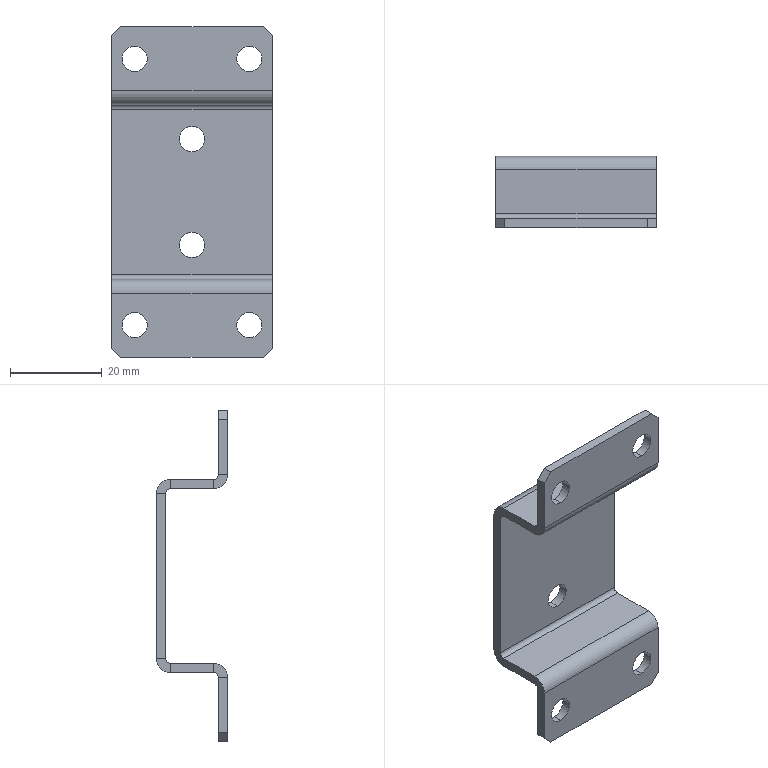Part | STEP file | HXGR200008-06-03-01 | 1 solid | 54 faces | box 35 x 15.5 x 72 mm | volume 6389 mm3 | plane 34 | cylinder 20 | commonest cylinder face diameters 5.5 x12 2 x4 6 x4
STEP:
#1=CARTESIAN_POINT('',(0.,5.75,10.25));
#2=VERTEX_POINT('',#1);
#3=CARTESIAN_POINT('',(0.,5.75,4.75));
#4=VERTEX_POINT('',#3);
#5=CARTESIAN_POINT('',(0.,5.75,7.5));
#6=DIRECTION('',(0.,-1.,0.));
#7=DIRECTION('',(0.,0.,-1.));
#8=AXIS2_PLACEMENT_3D('',#5,#6,#7);
#9=CIRCLE('',#8,2.75);
#10=EDGE_CURVE('',#2,#4,#9,.T.);
#11=ORIENTED_EDGE('',*,*,#10,.T.);
#12=CARTESIAN_POINT('',(0.,7.75,4.75));
#13=VERTEX_POINT('',#12);
#14=CARTESIAN_POINT('',(0.,7.75,4.75));
#15=DIRECTION('',(0.,1.,0.));
#16=VECTOR('',#15,1000.);
#17=LINE('',#14,#16);
#18=EDGE_CURVE('',#4,#13,#17,.T.);
#19=ORIENTED_EDGE('',*,*,#18,.T.);
#20=CARTESIAN_POINT('',(0.,7.75,10.25));
#21=VERTEX_POINT('',#20);
#22=CARTESIAN_POINT('',(0.,7.75,7.5));
#23=DIRECTION('',(0.,1.,0.));
#24=DIRECTION('',(0.,0.,1.));
#25=AXIS2_PLACEMENT_3D('',#22,#23,#24);
#26=CIRCLE('',#25,2.75);
#27=EDGE_CURVE('',#13,#21,#26,.T.);
#28=ORIENTED_EDGE('',*,*,#27,.T.);
#29=CARTESIAN_POINT('',(0.,7.75,10.25));
#30=DIRECTION('',(0.,1.,0.));
#31=VECTOR('',#30,1000.);
#32=LINE('',#29,#31);
#33=EDGE_CURVE('',#2,#21,#32,.T.);
#34=ORIENTED_EDGE('',*,*,#33,.F.);
#35=EDGE_LOOP('',(#11,#19,#28,#34));
#36=FACE_OUTER_BOUND('',#35,.T.);
#37=CARTESIAN_POINT('',(0.,7.75,7.5));
#38=DIRECTION('',(0.,1.,0.));
#39=DIRECTION('',(0.,0.,1.));
#40=AXIS2_PLACEMENT_3D('',#37,#38,#39);
#41=CYLINDRICAL_SURFACE('',#40,2.75);
#42=ADVANCED_FACE('',(#36),#41,.F.);
#43=CARTESIAN_POINT('',(0.,5.75,33.25));
#44=VERTEX_POINT('',#43);
#45=CARTESIAN_POINT('',(0.,5.75,27.75));
#46=VERTEX_POINT('',#45);
#47=CARTESIAN_POINT('',(0.,5.75,30.5));
#48=DIRECTION('',(0.,-1.,0.));
#49=DIRECTION('',(0.,0.,-1.));
#50=AXIS2_PLACEMENT_3D('',#47,#48,#49);
#51=CIRCLE('',#50,2.75);
#52=EDGE_CURVE('',#44,#46,#51,.T.);
#53=ORIENTED_EDGE('',*,*,#52,.T.);
#54=CARTESIAN_POINT('',(0.,7.75,27.75));
#55=VERTEX_POINT('',#54);
#56=CARTESIAN_POINT('',(0.,7.75,27.75));
#57=DIRECTION('',(0.,1.,0.));
#58=VECTOR('',#57,1000.);
#59=LINE('',#56,#58);
#60=EDGE_CURVE('',#46,#55,#59,.T.);
#61=ORIENTED_EDGE('',*,*,#60,.T.);
#62=CARTESIAN_POINT('',(0.,7.75,33.25));
#63=VERTEX_POINT('',#62);
#64=CARTESIAN_POINT('',(0.,7.75,30.5));
#65=DIRECTION('',(0.,1.,0.));
#66=DIRECTION('',(0.,0.,1.));
#67=AXIS2_PLACEMENT_3D('',#64,#65,#66);
#68=CIRCLE('',#67,2.75);
#69=EDGE_CURVE('',#55,#63,#68,.T.);
#70=ORIENTED_EDGE('',*,*,#69,.T.);
#71=CARTESIAN_POINT('',(0.,7.75,33.25));
#72=DIRECTION('',(0.,1.,0.));
#73=VECTOR('',#72,1000.);
#74=LINE('',#71,#73);
#75=EDGE_CURVE('',#44,#63,#74,.T.);
#76=ORIENTED_EDGE('',*,*,#75,.F.);
#77=EDGE_LOOP('',(#53,#61,#70,#76));
#78=FACE_OUTER_BOUND('',#77,.T.);
#79=CARTESIAN_POINT('',(0.,7.75,30.5));
#80=DIRECTION('',(0.,1.,0.));
#81=DIRECTION('',(0.,0.,1.));
#82=AXIS2_PLACEMENT_3D('',#79,#80,#81);
#83=CYLINDRICAL_SURFACE('',#82,2.75);
#84=ADVANCED_FACE('',(#78),#83,.F.);
#85=CARTESIAN_POINT('',(-12.5,-7.75,-7.25));
#86=VERTEX_POINT('',#85);
#87=CARTESIAN_POINT('',(-12.5,-7.75,-12.75));
#88=VERTEX_POINT('',#87);
#89=CARTESIAN_POINT('',(-12.5,-7.75,-10.));
#90=DIRECTION('',(0.,-1.,0.));
#91=DIRECTION('',(0.,0.,-1.));
#92=AXIS2_PLACEMENT_3D('',#89,#90,#91);
#93=CIRCLE('',#92,2.75);
#94=EDGE_CURVE('',#86,#88,#93,.T.);
#95=ORIENTED_EDGE('',*,*,#94,.T.);
#96=CARTESIAN_POINT('',(-12.5,-5.75,-12.75));
#97=VERTEX_POINT('',#96);
#98=CARTESIAN_POINT('',(-12.5,-5.75,-12.75));
#99=DIRECTION('',(0.,1.,0.));
#100=VECTOR('',#99,1000.);
#101=LINE('',#98,#100);
#102=EDGE_CURVE('',#88,#97,#101,.T.);
#103=ORIENTED_EDGE('',*,*,#102,.T.);
#104=CARTESIAN_POINT('',(-12.5,-5.75,-7.25));
#105=VERTEX_POINT('',#104);
#106=CARTESIAN_POINT('',(-12.5,-5.75,-10.));
#107=DIRECTION('',(0.,1.,0.));
#108=DIRECTION('',(0.,0.,1.));
#109=AXIS2_PLACEMENT_3D('',#106,#107,#108);
#110=CIRCLE('',#109,2.75);
#111=EDGE_CURVE('',#97,#105,#110,.T.);
#112=ORIENTED_EDGE('',*,*,#111,.T.);
#113=CARTESIAN_POINT('',(-12.5,-5.75,-7.25));
#114=DIRECTION('',(0.,1.,0.));
#115=VECTOR('',#114,1000.);
#116=LINE('',#113,#115);
#117=EDGE_CURVE('',#86,#105,#116,.T.);
#118=ORIENTED_EDGE('',*,*,#117,.F.);
#119=EDGE_LOOP('',(#95,#103,#112,#118));
#120=FACE_OUTER_BOUND('',#119,.T.);
#121=CARTESIAN_POINT('',(-12.5,-5.75,-10.));
#122=DIRECTION('',(0.,1.,0.));
#123=DIRECTION('',(0.,0.,1.));
#124=AXIS2_PLACEMENT_3D('',#121,#122,#123);
#125=CYLINDRICAL_SURFACE('',#124,2.75);
#126=ADVANCED_FACE('',(#120),#125,.F.);
#127=CARTESIAN_POINT('',(12.5,-7.75,-7.25));
#128=VERTEX_POINT('',#127);
#129=CARTESIAN_POINT('',(12.5,-7.75,-12.75));
#130=VERTEX_POINT('',#129);
#131=CARTESIAN_POINT('',(12.5,-7.75,-10.));
#132=DIRECTION('',(0.,-1.,0.));
#133=DIRECTION('',(0.,0.,-1.));
#134=AXIS2_PLACEMENT_3D('',#131,#132,#133);
#135=CIRCLE('',#134,2.75);
#136=EDGE_CURVE('',#128,#130,#135,.T.);
#137=ORIENTED_EDGE('',*,*,#136,.T.);
#138=CARTESIAN_POINT('',(12.5,-5.75,-12.75));
#139=VERTEX_POINT('',#138);
#140=CARTESIAN_POINT('',(12.5,-5.75,-12.75));
#141=DIRECTION('',(0.,1.,0.));
#142=VECTOR('',#141,1000.);
#143=LINE('',#140,#142);
#144=EDGE_CURVE('',#130,#139,#143,.T.);
#145=ORIENTED_EDGE('',*,*,#144,.T.);
#146=CARTESIAN_POINT('',(12.5,-5.75,-7.25));
#147=VERTEX_POINT('',#146);
#148=CARTESIAN_POINT('',(12.5,-5.75,-10.));
#149=DIRECTION('',(0.,1.,0.));
#150=DIRECTION('',(0.,0.,1.));
#151=AXIS2_PLACEMENT_3D('',#148,#149,#150);
#152=CIRCLE('',#151,2.75);
#153=EDGE_CURVE('',#139,#147,#152,.T.);
#154=ORIENTED_EDGE('',*,*,#153,.T.);
#155=CARTESIAN_POINT('',(12.5,-5.75,-7.25));
#156=DIRECTION('',(0.,1.,0.));
#157=VECTOR('',#156,1000.);
#158=LINE('',#155,#157);
#159=EDGE_CURVE('',#128,#147,#158,.T.);
#160=ORIENTED_EDGE('',*,*,#159,.F.);
#161=EDGE_LOOP('',(#137,#145,#154,#160));
#162=FACE_OUTER_BOUND('',#161,.T.);
#163=CARTESIAN_POINT('',(12.5,-5.75,-10.));
#164=DIRECTION('',(0.,1.,0.));
#165=DIRECTION('',(0.,0.,1.));
#166=AXIS2_PLACEMENT_3D('',#163,#164,#165);
#167=CYLINDRICAL_SURFACE('',#166,2.75);
#168=ADVANCED_FACE('',(#162),#167,.F.);
#169=CARTESIAN_POINT('',(-12.5,-7.75,45.25));
#170=VERTEX_POINT('',#169);
#171=CARTESIAN_POINT('',(-12.5,-7.75,50.75));
#172=VERTEX_POINT('',#171);
#173=CARTESIAN_POINT('',(-12.5,-7.75,48.));
#174=DIRECTION('',(0.,1.,0.));
#175=DIRECTION('',(0.,0.,1.));
#176=AXIS2_PLACEMENT_3D('',#173,#174,#175);
#177=CIRCLE('',#176,2.75);
#178=EDGE_CURVE('',#170,#172,#177,.T.);
#179=ORIENTED_EDGE('',*,*,#178,.F.);
#180=CARTESIAN_POINT('',(-12.5,-5.75,45.25));
#181=VERTEX_POINT('',#180);
#182=CARTESIAN_POINT('',(-12.5,-5.75,45.25));
#183=DIRECTION('',(0.,1.,0.));
#184=VECTOR('',#183,1000.);
#185=LINE('',#182,#184);
#186=EDGE_CURVE('',#170,#181,#185,.T.);
#187=ORIENTED_EDGE('',*,*,#186,.T.);
#188=CARTESIAN_POINT('',(-12.5,-5.75,50.75));
#189=VERTEX_POINT('',#188);
#190=CARTESIAN_POINT('',(-12.5,-5.75,48.));
#191=DIRECTION('',(0.,1.,0.));
#192=DIRECTION('',(0.,0.,1.));
#193=AXIS2_PLACEMENT_3D('',#190,#191,#192);
#194=CIRCLE('',#193,2.75);
#195=EDGE_CURVE('',#181,#189,#194,.T.);
#196=ORIENTED_EDGE('',*,*,#195,.T.);
#197=CARTESIAN_POINT('',(-12.5,-5.75,50.75));
#198=DIRECTION('',(0.,1.,0.));
#199=VECTOR('',#198,1000.);
#200=LINE('',#197,#199);
#201=EDGE_CURVE('',#172,#189,#200,.T.);
#202=ORIENTED_EDGE('',*,*,#201,.F.);
#203=EDGE_LOOP('',(#179,#187,#196,#202));
#204=FACE_OUTER_BOUND('',#203,.T.);
#205=CARTESIAN_POINT('',(-12.5,-5.75,48.));
#206=DIRECTION('',(0.,1.,0.));
#207=DIRECTION('',(0.,0.,1.));
#208=AXIS2_PLACEMENT_3D('',#205,#206,#207);
#209=CYLINDRICAL_SURFACE('',#208,2.75);
#210=ADVANCED_FACE('',(#204),#209,.F.);
#211=CARTESIAN_POINT('',(12.5,-7.75,45.25));
#212=VERTEX_POINT('',#211);
#213=CARTESIAN_POINT('',(12.5,-7.75,50.75));
#214=VERTEX_POINT('',#213);
#215=CARTESIAN_POINT('',(12.5,-7.75,48.));
#216=DIRECTION('',(0.,1.,0.));
#217=DIRECTION('',(0.,0.,1.));
#218=AXIS2_PLACEMENT_3D('',#215,#216,#217);
#219=CIRCLE('',#218,2.75);
#220=EDGE_CURVE('',#212,#214,#219,.T.);
#221=ORIENTED_EDGE('',*,*,#220,.F.);
#222=CARTESIAN_POINT('',(12.5,-5.75,45.25));
#223=VERTEX_POINT('',#222);
#224=CARTESIAN_POINT('',(12.5,-5.75,45.25));
#225=DIRECTION('',(0.,1.,0.));
#226=VECTOR('',#225,1000.);
#227=LINE('',#224,#226);
#228=EDGE_CURVE('',#212,#223,#227,.T.);
#229=ORIENTED_EDGE('',*,*,#228,.T.);
#230=CARTESIAN_POINT('',(12.5,-5.75,50.75));
#231=VERTEX_POINT('',#230);
#232=CARTESIAN_POINT('',(12.5,-5.75,48.));
#233=DIRECTION('',(0.,1.,0.));
#234=DIRECTION('',(0.,0.,1.));
#235=AXIS2_PLACEMENT_3D('',#232,#233,#234);
#236=CIRCLE('',#235,2.75);
#237=EDGE_CURVE('',#223,#231,#236,.T.);
#238=ORIENTED_EDGE('',*,*,#237,.T.);
#239=CARTESIAN_POINT('',(12.5,-5.75,50.75));
#240=DIRECTION('',(0.,1.,0.));
#241=VECTOR('',#240,1000.);
#242=LINE('',#239,#241);
#243=EDGE_CURVE('',#214,#231,#242,.T.);
#244=ORIENTED_EDGE('',*,*,#243,.F.);
#245=EDGE_LOOP('',(#221,#229,#238,#244));
#246=FACE_OUTER_BOUND('',#245,.T.);
#247=CARTESIAN_POINT('',(12.5,-5.75,48.));
#248=DIRECTION('',(0.,1.,0.));
#249=DIRECTION('',(0.,0.,1.));
#250=AXIS2_PLACEMENT_3D('',#247,#248,#249);
#251=CYLINDRICAL_SURFACE('',#250,2.75);
#252=ADVANCED_FACE('',(#246),#251,.F.);
#253=CARTESIAN_POINT('',(-12.5,-5.75,-10.));
#254=DIRECTION('',(0.,1.,0.));
#255=DIRECTION('',(0.,0.,1.));
#256=AXIS2_PLACEMENT_3D('',#253,#254,#255);
#257=CIRCLE('',#256,2.75);
#258=EDGE_CURVE('',#105,#97,#257,.T.);
#259=ORIENTED_EDGE('',*,*,#258,.F.);
#260=ORIENTED_EDGE('',*,*,#111,.F.);
#261=EDGE_LOOP('',(#259,#260));
#262=FACE_BOUND('',#261,.T.);
#263=CARTESIAN_POINT('',(15.5,-5.75,-17.));
#264=VERTEX_POINT('',#263);
#265=CARTESIAN_POINT('',(-15.5,-5.75,-17.));
#266=VERTEX_POINT('',#265);
#267=CARTESIAN_POINT('',(0.,-5.75,-17.));
#268=DIRECTION('',(-1.,0.,0.));
#269=VECTOR('',#268,1000.);
#270=LINE('',#267,#269);
#271=EDGE_CURVE('',#264,#266,#270,.T.);
#272=ORIENTED_EDGE('',*,*,#271,.T.);
#273=CARTESIAN_POINT('',(-17.5,-5.75,-15.));
#274=VERTEX_POINT('',#273);
#275=CARTESIAN_POINT('',(-15.5,-5.75,-17.));
#276=DIRECTION('',(-0.7071,0.,0.7071));
#277=VECTOR('',#276,1000.);
#278=LINE('',#275,#277);
#279=EDGE_CURVE('',#266,#274,#278,.T.);
#280=ORIENTED_EDGE('',*,*,#279,.T.);
#281=CARTESIAN_POINT('',(-17.5,-5.75,-3.));
#282=VERTEX_POINT('',#281);
#283=CARTESIAN_POINT('',(-17.5,-5.75,0.));
#284=DIRECTION('',(0.,0.,1.));
#285=VECTOR('',#284,1000.);
#286=LINE('',#283,#285);
#287=EDGE_CURVE('',#274,#282,#286,.T.);
#288=ORIENTED_EDGE('',*,*,#287,.T.);
#289=CARTESIAN_POINT('',(17.5,-5.75,-3.));
#290=VERTEX_POINT('',#289);
#291=CARTESIAN_POINT('',(17.5,-5.75,-3.));
#292=DIRECTION('',(-1.,0.,0.));
#293=VECTOR('',#292,1000.);
#294=LINE('',#291,#293);
#295=EDGE_CURVE('',#290,#282,#294,.T.);
#296=ORIENTED_EDGE('',*,*,#295,.F.);
#297=CARTESIAN_POINT('',(17.5,-5.75,-15.));
#298=VERTEX_POINT('',#297);
#299=CARTESIAN_POINT('',(17.5,-5.75,0.));
#300=DIRECTION('',(0.,0.,-1.));
#301=VECTOR('',#300,1000.);
#302=LINE('',#299,#301);
#303=EDGE_CURVE('',#290,#298,#302,.T.);
#304=ORIENTED_EDGE('',*,*,#303,.T.);
#305=CARTESIAN_POINT('',(17.5,-5.75,-15.));
#306=DIRECTION('',(-0.7071,0.,-0.7071));
#307=VECTOR('',#306,1000.);
#308=LINE('',#305,#307);
#309=EDGE_CURVE('',#298,#264,#308,.T.);
#310=ORIENTED_EDGE('',*,*,#309,.T.);
#311=EDGE_LOOP('',(#272,#280,#288,#296,#304,#310));
#312=FACE_OUTER_BOUND('',#311,.T.);
#313=CARTESIAN_POINT('',(12.5,-5.75,-10.));
#314=DIRECTION('',(0.,1.,0.));
#315=DIRECTION('',(0.,0.,1.));
#316=AXIS2_PLACEMENT_3D('',#313,#314,#315);
#317=CIRCLE('',#316,2.75);
#318=EDGE_CURVE('',#147,#139,#317,.T.);
#319=ORIENTED_EDGE('',*,*,#318,.F.);
#320=ORIENTED_EDGE('',*,*,#153,.F.);
#321=EDGE_LOOP('',(#319,#320));
#322=FACE_BOUND('',#321,.T.);
#323=CARTESIAN_POINT('',(0.,-5.75,0.));
#324=DIRECTION('',(0.,-1.,0.));
#325=DIRECTION('',(0.,0.,-1.));
#326=AXIS2_PLACEMENT_3D('',#323,#324,#325);
#327=PLANE('',#326);
#328=ADVANCED_FACE('',(#262,#312,#322),#327,.F.);
#329=CARTESIAN_POINT('',(-17.5,-4.75,40.));
#330=VERTEX_POINT('',#329);
#331=CARTESIAN_POINT('',(-17.5,-4.75,38.));
#332=VERTEX_POINT('',#331);
#333=CARTESIAN_POINT('',(-17.5,-4.75,40.));
#334=DIRECTION('',(0.,0.,-1.));
#335=VECTOR('',#334,1000.);
#336=LINE('',#333,#335);
#337=EDGE_CURVE('',#330,#332,#336,.T.);
#338=ORIENTED_EDGE('',*,*,#337,.F.);
#339=CARTESIAN_POINT('',(-17.5,4.75,40.));
#340=VERTEX_POINT('',#339);
#341=CARTESIAN_POINT('',(-17.5,0.,40.));
#342=DIRECTION('',(0.,-1.,0.));
#343=VECTOR('',#342,1000.);
#344=LINE('',#341,#343);
#345=EDGE_CURVE('',#340,#330,#344,.T.);
#346=ORIENTED_EDGE('',*,*,#345,.F.);
#347=CARTESIAN_POINT('',(-17.5,4.75,38.));
#348=VERTEX_POINT('',#347);
#349=CARTESIAN_POINT('',(-17.5,4.75,38.));
#350=DIRECTION('',(0.,0.,1.));
#351=VECTOR('',#350,1000.);
#352=LINE('',#349,#351);
#353=EDGE_CURVE('',#348,#340,#352,.T.);
#354=ORIENTED_EDGE('',*,*,#353,.F.);
#355=CARTESIAN_POINT('',(-17.5,-7.75,38.));
#356=DIRECTION('',(0.,-1.,0.));
#357=VECTOR('',#356,1000.);
#358=LINE('',#355,#357);
#359=EDGE_CURVE('',#348,#332,#358,.T.);
#360=ORIENTED_EDGE('',*,*,#359,.T.);
#361=EDGE_LOOP('',(#338,#346,#354,#360));
#362=FACE_OUTER_BOUND('',#361,.T.);
#363=CARTESIAN_POINT('',(-17.5,-7.75,40.));
#364=DIRECTION('',(1.,0.,0.));
#365=DIRECTION('',(0.,0.,-1.));
#366=AXIS2_PLACEMENT_3D('',#363,#364,#365);
#367=PLANE('',#366);
#368=ADVANCED_FACE('',(#362),#367,.F.);
#369=CARTESIAN_POINT('',(17.5,-4.75,40.));
#370=VERTEX_POINT('',#369);
#371=CARTESIAN_POINT('',(17.5,-4.75,38.));
#372=VERTEX_POINT('',#371);
#373=CARTESIAN_POINT('',(17.5,-4.75,40.));
#374=DIRECTION('',(0.,0.,-1.));
#375=VECTOR('',#374,1000.);
#376=LINE('',#373,#375);
#377=EDGE_CURVE('',#370,#372,#376,.T.);
#378=ORIENTED_EDGE('',*,*,#377,.T.);
#379=CARTESIAN_POINT('',(17.5,4.75,38.));
#380=VERTEX_POINT('',#379);
#381=CARTESIAN_POINT('',(17.5,5.75,38.));
#382=DIRECTION('',(0.,1.,0.));
#383=VECTOR('',#382,1000.);
#384=LINE('',#381,#383);
#385=EDGE_CURVE('',#372,#380,#384,.T.);
#386=ORIENTED_EDGE('',*,*,#385,.T.);
#387=CARTESIAN_POINT('',(17.5,4.75,40.));
#388=VERTEX_POINT('',#387);
#389=CARTESIAN_POINT('',(17.5,4.75,40.));
#390=DIRECTION('',(0.,0.,1.));
#391=VECTOR('',#390,1000.);
#392=LINE('',#389,#391);
#393=EDGE_CURVE('',#380,#388,#392,.T.);
#394=ORIENTED_EDGE('',*,*,#393,.T.);
#395=CARTESIAN_POINT('',(17.5,0.,40.));
#396=DIRECTION('',(0.,1.,0.));
#397=VECTOR('',#396,1000.);
#398=LINE('',#395,#397);
#399=EDGE_CURVE('',#370,#388,#398,.T.);
#400=ORIENTED_EDGE('',*,*,#399,.F.);
#401=EDGE_LOOP('',(#378,#386,#394,#400));
#402=FACE_OUTER_BOUND('',#401,.T.);
#403=CARTESIAN_POINT('',(17.5,5.75,40.));
#404=DIRECTION('',(-1.,0.,0.));
#405=DIRECTION('',(0.,0.,1.));
#406=AXIS2_PLACEMENT_3D('',#403,#404,#405);
#407=PLANE('',#406);
#408=ADVANCED_FACE('',(#402),#407,.F.);
#409=CARTESIAN_POINT('',(17.5,-4.75,40.));
#410=DIRECTION('',(-1.,0.,0.));
#411=VECTOR('',#410,1000.);
#412=LINE('',#409,#411);
#413=EDGE_CURVE('',#370,#330,#412,.T.);
#414=ORIENTED_EDGE('',*,*,#413,.F.);
#415=ORIENTED_EDGE('',*,*,#399,.T.);
#416=CARTESIAN_POINT('',(17.5,4.75,40.));
#417=DIRECTION('',(1.,0.,0.));
#418=VECTOR('',#417,1000.);
#419=LINE('',#416,#418);
#420=EDGE_CURVE('',#340,#388,#419,.T.);
#421=ORIENTED_EDGE('',*,*,#420,.F.);
#422=ORIENTED_EDGE('',*,*,#345,.T.);
#423=EDGE_LOOP('',(#414,#415,#421,#422));
#424=FACE_OUTER_BOUND('',#423,.T.);
#425=CARTESIAN_POINT('',(0.,0.,40.));
#426=DIRECTION('',(0.,0.,-1.));
#427=DIRECTION('',(0.,1.,0.));
#428=AXIS2_PLACEMENT_3D('',#425,#426,#427);
#429=PLANE('',#428);
#430=ADVANCED_FACE('',(#424),#429,.F.);
#431=ORIENTED_EDGE('',*,*,#385,.F.);
#432=CARTESIAN_POINT('',(17.5,-4.75,38.));
#433=DIRECTION('',(-1.,0.,0.));
#434=VECTOR('',#433,1000.);
#435=LINE('',#432,#434);
#436=EDGE_CURVE('',#372,#332,#435,.T.);
#437=ORIENTED_EDGE('',*,*,#436,.T.);
#438=ORIENTED_EDGE('',*,*,#359,.F.);
#439=CARTESIAN_POINT('',(17.5,4.75,38.));
#440=DIRECTION('',(-1.,0.,0.));
#441=VECTOR('',#440,1000.);
#442=LINE('',#439,#441);
#443=EDGE_CURVE('',#380,#348,#442,.T.);
#444=ORIENTED_EDGE('',*,*,#443,.F.);
#445=EDGE_LOOP('',(#431,#437,#438,#444));
#446=FACE_OUTER_BOUND('',#445,.T.);
#447=CARTESIAN_POINT('',(0.,0.,38.));
#448=DIRECTION('',(0.,0.,-1.));
#449=DIRECTION('',(0.,1.,0.));
#450=AXIS2_PLACEMENT_3D('',#447,#448,#449);
#451=PLANE('',#450);
#452=ADVANCED_FACE('',(#446),#451,.T.);
#453=CARTESIAN_POINT('',(17.5,5.75,37.));
#454=VERTEX_POINT('',#453);
#455=CARTESIAN_POINT('',(17.5,7.75,37.));
#456=VERTEX_POINT('',#455);
#457=CARTESIAN_POINT('',(17.5,5.75,37.));
#458=DIRECTION('',(0.,1.,0.));
#459=VECTOR('',#458,1000.);
#460=LINE('',#457,#459);
#461=EDGE_CURVE('',#454,#456,#460,.T.);
#462=ORIENTED_EDGE('',*,*,#461,.F.);
#463=CARTESIAN_POINT('',(17.5,5.75,1.));
#464=VERTEX_POINT('',#463);
#465=CARTESIAN_POINT('',(17.5,5.75,0.));
#466=DIRECTION('',(0.,0.,-1.));
#467=VECTOR('',#466,1000.);
#468=LINE('',#465,#467);
#469=EDGE_CURVE('',#454,#464,#468,.T.);
#470=ORIENTED_EDGE('',*,*,#469,.T.);
#471=CARTESIAN_POINT('',(17.5,7.75,1.));
#472=VERTEX_POINT('',#471);
#473=CARTESIAN_POINT('',(17.5,7.75,1.));
#474=DIRECTION('',(0.,1.,0.));
#475=VECTOR('',#474,1000.);
#476=LINE('',#473,#475);
#477=EDGE_CURVE('',#464,#472,#476,.T.);
#478=ORIENTED_EDGE('',*,*,#477,.T.);
#479=CARTESIAN_POINT('',(17.5,7.75,0.));
#480=DIRECTION('',(0.,0.,-1.));
#481=VECTOR('',#480,1000.);
#482=LINE('',#479,#481);
#483=EDGE_CURVE('',#456,#472,#482,.T.);
#484=ORIENTED_EDGE('',*,*,#483,.F.);
#485=EDGE_LOOP('',(#462,#470,#478,#484));
#486=FACE_OUTER_BOUND('',#485,.T.);
#487=CARTESIAN_POINT('',(17.5,7.75,0.));
#488=DIRECTION('',(-1.,0.,0.));
#489=DIRECTION('',(0.,0.,1.));
#490=AXIS2_PLACEMENT_3D('',#487,#488,#489);
#491=PLANE('',#490);
#492=ADVANCED_FACE('',(#486),#491,.F.);
#493=CARTESIAN_POINT('',(-17.5,5.75,37.));
#494=VERTEX_POINT('',#493);
#495=CARTESIAN_POINT('',(-17.5,7.75,37.));
#496=VERTEX_POINT('',#495);
#497=CARTESIAN_POINT('',(-17.5,5.75,37.));
#498=DIRECTION('',(0.,1.,0.));
#499=VECTOR('',#498,1000.);
#500=LINE('',#497,#499);
#501=EDGE_CURVE('',#494,#496,#500,.T.);
#502=ORIENTED_EDGE('',*,*,#501,.T.);
#503=CARTESIAN_POINT('',(-17.5,7.75,1.));
#504=VERTEX_POINT('',#503);
#505=CARTESIAN_POINT('',(-17.5,7.75,0.));
#506=DIRECTION('',(0.,0.,1.));
#507=VECTOR('',#506,1000.);
#508=LINE('',#505,#507);
#509=EDGE_CURVE('',#504,#496,#508,.T.);
#510=ORIENTED_EDGE('',*,*,#509,.F.);
#511=CARTESIAN_POINT('',(-17.5,5.75,1.));
#512=VERTEX_POINT('',#511);
#513=CARTESIAN_POINT('',(-17.5,5.75,1.));
#514=DIRECTION('',(0.,1.,0.));
#515=VECTOR('',#514,1000.);
#516=LINE('',#513,#515);
#517=EDGE_CURVE('',#512,#504,#516,.T.);
#518=ORIENTED_EDGE('',*,*,#517,.F.);
#519=CARTESIAN_POINT('',(-17.5,5.75,40.));
#520=DIRECTION('',(0.,0.,1.));
#521=VECTOR('',#520,1000.);
#522=LINE('',#519,#521);
#523=EDGE_CURVE('',#512,#494,#522,.T.);
#524=ORIENTED_EDGE('',*,*,#523,.T.);
#525=EDGE_LOOP('',(#502,#510,#518,#524));
#526=FACE_OUTER_BOUND('',#525,.T.);
#527=CARTESIAN_POINT('',(-17.5,7.75,40.));
#528=DIRECTION('',(1.,0.,0.));
#529=DIRECTION('',(0.,0.,-1.));
#530=AXIS2_PLACEMENT_3D('',#527,#528,#529);
#531=PLANE('',#530);
#532=ADVANCED_FACE('',(#526),#531,.F.);
#533=CARTESIAN_POINT('',(0.,7.75,7.5));
#534=DIRECTION('',(0.,1.,0.));
#535=DIRECTION('',(0.,0.,1.));
#536=AXIS2_PLACEMENT_3D('',#533,#534,#535);
#537=CIRCLE('',#536,2.75);
#538=EDGE_CURVE('',#21,#13,#537,.T.);
#539=ORIENTED_EDGE('',*,*,#538,.F.);
#540=ORIENTED_EDGE('',*,*,#27,.F.);
#541=EDGE_LOOP('',(#539,#540));
#542=FACE_BOUND('',#541,.T.);
#543=CARTESIAN_POINT('',(0.,7.75,30.5));
#544=DIRECTION('',(0.,1.,0.));
#545=DIRECTION('',(0.,0.,1.));
#546=AXIS2_PLACEMENT_3D('',#543,#544,#545);
#547=CIRCLE('',#546,2.75);
#548=EDGE_CURVE('',#63,#55,#547,.T.);
#549=ORIENTED_EDGE('',*,*,#548,.F.);
#550=ORIENTED_EDGE('',*,*,#69,.F.);
#551=EDGE_LOOP('',(#549,#550));
#552=FACE_BOUND('',#551,.T.);
#553=CARTESIAN_POINT('',(-17.5,7.75,37.));
#554=DIRECTION('',(1.,0.,0.));
#555=VECTOR('',#554,1000.);
#556=LINE('',#553,#555);
#557=EDGE_CURVE('',#496,#456,#556,.T.);
#558=ORIENTED_EDGE('',*,*,#557,.T.);
#559=ORIENTED_EDGE('',*,*,#483,.T.);
#560=CARTESIAN_POINT('',(17.5,7.75,1.));
#561=DIRECTION('',(1.,0.,0.));
#562=VECTOR('',#561,1000.);
#563=LINE('',#560,#562);
#564=EDGE_CURVE('',#504,#472,#563,.T.);
#565=ORIENTED_EDGE('',*,*,#564,.F.);
#566=ORIENTED_EDGE('',*,*,#509,.T.);
#567=EDGE_LOOP('',(#558,#559,#565,#566));
#568=FACE_OUTER_BOUND('',#567,.T.);
#569=CARTESIAN_POINT('',(0.,7.75,0.));
#570=DIRECTION('',(0.,-1.,0.));
#571=DIRECTION('',(0.,0.,-1.));
#572=AXIS2_PLACEMENT_3D('',#569,#570,#571);
#573=PLANE('',#572);
#574=ADVANCED_FACE('',(#542,#552,#568),#573,.F.);
#575=ORIENTED_EDGE('',*,*,#10,.F.);
#576=CARTESIAN_POINT('',(0.,5.75,7.5));
#577=DIRECTION('',(0.,-1.,0.));
#578=DIRECTION('',(0.,0.,-1.));
#579=AXIS2_PLACEMENT_3D('',#576,#577,#578);
#580=CIRCLE('',#579,2.75);
#581=EDGE_CURVE('',#4,#2,#580,.T.);
#582=ORIENTED_EDGE('',*,*,#581,.F.);
#583=EDGE_LOOP('',(#575,#582));
#584=FACE_BOUND('',#583,.T.);
#585=ORIENTED_EDGE('',*,*,#52,.F.);
#586=CARTESIAN_POINT('',(0.,5.75,30.5));
#587=DIRECTION('',(0.,-1.,0.));
#588=DIRECTION('',(0.,0.,-1.));
#589=AXIS2_PLACEMENT_3D('',#586,#587,#588);
#590=CIRCLE('',#589,2.75);
#591=EDGE_CURVE('',#46,#44,#590,.T.);
#592=ORIENTED_EDGE('',*,*,#591,.F.);
#593=EDGE_LOOP('',(#585,#592));
#594=FACE_BOUND('',#593,.T.);
#595=ORIENTED_EDGE('',*,*,#469,.F.);
#596=CARTESIAN_POINT('',(-17.5,5.75,37.));
#597=DIRECTION('',(1.,0.,0.));
#598=VECTOR('',#597,1000.);
#599=LINE('',#596,#598);
#600=EDGE_CURVE('',#494,#454,#599,.T.);
#601=ORIENTED_EDGE('',*,*,#600,.F.);
#602=ORIENTED_EDGE('',*,*,#523,.F.);
#603=CARTESIAN_POINT('',(17.5,5.75,1.));
#604=DIRECTION('',(-1.,0.,0.));
#605=VECTOR('',#604,1000.);
#606=LINE('',#603,#605);
#607=EDGE_CURVE('',#464,#512,#606,.T.);
#608=ORIENTED_EDGE('',*,*,#607,.F.);
#609=EDGE_LOOP('',(#595,#601,#602,#608));
#610=FACE_OUTER_BOUND('',#609,.T.);
#611=CARTESIAN_POINT('',(0.,5.75,0.));
#612=DIRECTION('',(0.,-1.,0.));
#613=DIRECTION('',(0.,0.,-1.));
#614=AXIS2_PLACEMENT_3D('',#611,#612,#613);
#615=PLANE('',#614);
#616=ADVANCED_FACE('',(#584,#594,#610),#615,.T.);
#617=CARTESIAN_POINT('',(-17.5,4.75,0.));
#618=VERTEX_POINT('',#617);
#619=CARTESIAN_POINT('',(-17.5,-4.75,0.));
#620=VERTEX_POINT('',#619);
#621=CARTESIAN_POINT('',(-17.5,7.75,0.));
#622=DIRECTION('',(0.,-1.,0.));
#623=VECTOR('',#622,1000.);
#624=LINE('',#621,#623);
#625=EDGE_CURVE('',#618,#620,#624,.T.);
#626=ORIENTED_EDGE('',*,*,#625,.F.);
#627=CARTESIAN_POINT('',(-17.5,4.75,-2.));
#628=VERTEX_POINT('',#627);
#629=CARTESIAN_POINT('',(-17.5,4.75,0.));
#630=DIRECTION('',(0.,0.,-1.));
#631=VECTOR('',#630,1000.);
#632=LINE('',#629,#631);
#633=EDGE_CURVE('',#618,#628,#632,.T.);
#634=ORIENTED_EDGE('',*,*,#633,.T.);
#635=CARTESIAN_POINT('',(-17.5,-4.75,-2.));
#636=VERTEX_POINT('',#635);
#637=CARTESIAN_POINT('',(-17.5,7.75,-2.));
#638=DIRECTION('',(0.,-1.,0.));
#639=VECTOR('',#638,1000.);
#640=LINE('',#637,#639);
#641=EDGE_CURVE('',#628,#636,#640,.T.);
#642=ORIENTED_EDGE('',*,*,#641,.T.);
#643=CARTESIAN_POINT('',(-17.5,-4.75,-2.));
#644=DIRECTION('',(0.,0.,1.));
#645=VECTOR('',#644,1000.);
#646=LINE('',#643,#645);
#647=EDGE_CURVE('',#636,#620,#646,.T.);
#648=ORIENTED_EDGE('',*,*,#647,.T.);
#649=EDGE_LOOP('',(#626,#634,#642,#648));
#650=FACE_OUTER_BOUND('',#649,.T.);
#651=CARTESIAN_POINT('',(-17.5,7.75,-2.));
#652=DIRECTION('',(-1.,0.,0.));
#653=DIRECTION('',(0.,-1.,0.));
#654=AXIS2_PLACEMENT_3D('',#651,#652,#653);
#655=PLANE('',#654);
#656=ADVANCED_FACE('',(#650),#655,.T.);
#657=CARTESIAN_POINT('',(17.5,4.75,-2.));
#658=VERTEX_POINT('',#657);
#659=CARTESIAN_POINT('',(-17.5,4.75,-2.));
#660=DIRECTION('',(1.,0.,0.));
#661=VECTOR('',#660,1000.);
#662=LINE('',#659,#661);
#663=EDGE_CURVE('',#628,#658,#662,.T.);
#664=ORIENTED_EDGE('',*,*,#663,.T.);
#665=CARTESIAN_POINT('',(17.5,-4.75,-2.));
#666=VERTEX_POINT('',#665);
#667=CARTESIAN_POINT('',(17.5,7.75,-2.));
#668=DIRECTION('',(0.,1.,0.));
#669=VECTOR('',#668,1000.);
#670=LINE('',#667,#669);
#671=EDGE_CURVE('',#666,#658,#670,.T.);
#672=ORIENTED_EDGE('',*,*,#671,.F.);
#673=CARTESIAN_POINT('',(-17.5,-4.75,-2.));
#674=DIRECTION('',(1.,0.,0.));
#675=VECTOR('',#674,1000.);
#676=LINE('',#673,#675);
#677=EDGE_CURVE('',#636,#666,#676,.T.);
#678=ORIENTED_EDGE('',*,*,#677,.F.);
#679=ORIENTED_EDGE('',*,*,#641,.F.);
#680=EDGE_LOOP('',(#664,#672,#678,#679));
#681=FACE_OUTER_BOUND('',#680,.T.);
#682=CARTESIAN_POINT('',(0.,0.,-2.));
#683=DIRECTION('',(0.,0.,1.));
#684=DIRECTION('',(1.,0.,0.));
#685=AXIS2_PLACEMENT_3D('',#682,#683,#684);
#686=PLANE('',#685);
#687=ADVANCED_FACE('',(#681),#686,.F.);
#688=CARTESIAN_POINT('',(17.5,-4.75,0.));
#689=VERTEX_POINT('',#688);
#690=CARTESIAN_POINT('',(17.5,4.75,0.));
#691=VERTEX_POINT('',#690);
#692=CARTESIAN_POINT('',(17.5,7.75,0.));
#693=DIRECTION('',(0.,1.,0.));
#694=VECTOR('',#693,1000.);
#695=LINE('',#692,#694);
#696=EDGE_CURVE('',#689,#691,#695,.T.);
#697=ORIENTED_EDGE('',*,*,#696,.T.);
#698=CARTESIAN_POINT('',(-17.5,4.75,0.));
#699=DIRECTION('',(1.,0.,0.));
#700=VECTOR('',#699,1000.);
#701=LINE('',#698,#700);
#702=EDGE_CURVE('',#618,#691,#701,.T.);
#703=ORIENTED_EDGE('',*,*,#702,.F.);
#704=ORIENTED_EDGE('',*,*,#625,.T.);
#705=CARTESIAN_POINT('',(-17.5,-4.75,0.));
#706=DIRECTION('',(1.,0.,0.));
#707=VECTOR('',#706,1000.);
#708=LINE('',#705,#707);
#709=EDGE_CURVE('',#620,#689,#708,.T.);
#710=ORIENTED_EDGE('',*,*,#709,.T.);
#711=EDGE_LOOP('',(#697,#703,#704,#710));
#712=FACE_OUTER_BOUND('',#711,.T.);
#713=CARTESIAN_POINT('',(0.,0.,0.));
#714=DIRECTION('',(0.,0.,1.));
#715=DIRECTION('',(1.,0.,0.));
#716=AXIS2_PLACEMENT_3D('',#713,#714,#715);
#717=PLANE('',#716);
#718=ADVANCED_FACE('',(#712),#717,.T.);
#719=CARTESIAN_POINT('',(17.5,4.75,0.));
#720=DIRECTION('',(0.,0.,-1.));
#721=VECTOR('',#720,1000.);
#722=LINE('',#719,#721);
#723=EDGE_CURVE('',#691,#658,#722,.T.);
#724=ORIENTED_EDGE('',*,*,#723,.F.);
#725=ORIENTED_EDGE('',*,*,#696,.F.);
#726=CARTESIAN_POINT('',(17.5,-4.75,-2.));
#727=DIRECTION('',(0.,0.,1.));
#728=VECTOR('',#727,1000.);
#729=LINE('',#726,#728);
#730=EDGE_CURVE('',#666,#689,#729,.T.);
#731=ORIENTED_EDGE('',*,*,#730,.F.);
#732=ORIENTED_EDGE('',*,*,#671,.T.);
#733=EDGE_LOOP('',(#724,#725,#731,#732));
#734=FACE_OUTER_BOUND('',#733,.T.);
#735=CARTESIAN_POINT('',(17.5,7.75,-2.));
#736=DIRECTION('',(1.,0.,0.));
#737=DIRECTION('',(0.,1.,0.));
#738=AXIS2_PLACEMENT_3D('',#735,#736,#737);
#739=PLANE('',#738);
#740=ADVANCED_FACE('',(#734),#739,.T.);
#741=CARTESIAN_POINT('',(17.5,-7.75,-3.));
#742=VERTEX_POINT('',#741);
#743=CARTESIAN_POINT('',(17.5,-7.75,-3.));
#744=DIRECTION('',(0.,-1.,0.));
#745=VECTOR('',#744,1000.);
#746=LINE('',#743,#745);
#747=EDGE_CURVE('',#290,#742,#746,.T.);
#748=ORIENTED_EDGE('',*,*,#747,.F.);
#749=CARTESIAN_POINT('',(17.5,-4.75,-3.));
#750=DIRECTION('',(1.,0.,0.));
#751=DIRECTION('',(0.,0.,1.));
#752=AXIS2_PLACEMENT_3D('',#749,#750,#751);
#753=CIRCLE('',#752,1.);
#754=EDGE_CURVE('',#666,#290,#753,.T.);
#755=ORIENTED_EDGE('',*,*,#754,.F.);
#756=ORIENTED_EDGE('',*,*,#730,.T.);
#757=CARTESIAN_POINT('',(17.5,-4.75,-3.));
#758=DIRECTION('',(1.,0.,0.));
#759=DIRECTION('',(0.,0.,1.));
#760=AXIS2_PLACEMENT_3D('',#757,#758,#759);
#761=CIRCLE('',#760,3.);
#762=EDGE_CURVE('',#689,#742,#761,.T.);
#763=ORIENTED_EDGE('',*,*,#762,.T.);
#764=EDGE_LOOP('',(#748,#755,#756,#763));
#765=FACE_OUTER_BOUND('',#764,.T.);
#766=CARTESIAN_POINT('',(17.5,-4.75,-3.));
#767=DIRECTION('',(1.,0.,0.));
#768=DIRECTION('',(0.,0.,-1.));
#769=AXIS2_PLACEMENT_3D('',#766,#767,#768);
#770=PLANE('',#769);
#771=ADVANCED_FACE('',(#765),#770,.T.);
#772=CARTESIAN_POINT('',(-17.5,-4.75,-3.));
#773=DIRECTION('',(-1.,0.,0.));
#774=DIRECTION('',(0.,0.,1.));
#775=AXIS2_PLACEMENT_3D('',#772,#773,#774);
#776=CIRCLE('',#775,1.);
#777=EDGE_CURVE('',#282,#636,#776,.T.);
#778=ORIENTED_EDGE('',*,*,#777,.F.);
#779=CARTESIAN_POINT('',(-17.5,-7.75,-3.));
#780=VERTEX_POINT('',#779);
#781=CARTESIAN_POINT('',(-17.5,-5.75,-3.));
#782=DIRECTION('',(0.,-1.,0.));
#783=VECTOR('',#782,1000.);
#784=LINE('',#781,#783);
#785=EDGE_CURVE('',#282,#780,#784,.T.);
#786=ORIENTED_EDGE('',*,*,#785,.T.);
#787=CARTESIAN_POINT('',(-17.5,-4.75,-3.));
#788=DIRECTION('',(-1.,0.,0.));
#789=DIRECTION('',(0.,0.,1.));
#790=AXIS2_PLACEMENT_3D('',#787,#788,#789);
#791=CIRCLE('',#790,3.);
#792=EDGE_CURVE('',#780,#620,#791,.T.);
#793=ORIENTED_EDGE('',*,*,#792,.T.);
#794=ORIENTED_EDGE('',*,*,#647,.F.);
#795=EDGE_LOOP('',(#778,#786,#793,#794));
#796=FACE_OUTER_BOUND('',#795,.T.);
#797=CARTESIAN_POINT('',(-17.5,-4.75,-3.));
#798=DIRECTION('',(1.,0.,0.));
#799=DIRECTION('',(0.,0.,-1.));
#800=AXIS2_PLACEMENT_3D('',#797,#798,#799);
#801=PLANE('',#800);
#802=ADVANCED_FACE('',(#796),#801,.F.);
#803=ORIENTED_EDGE('',*,*,#709,.F.);
#804=ORIENTED_EDGE('',*,*,#792,.F.);
#805=CARTESIAN_POINT('',(0.,-7.75,-3.));
#806=DIRECTION('',(-1.,0.,0.));
#807=VECTOR('',#806,1000.);
#808=LINE('',#805,#807);
#809=EDGE_CURVE('',#742,#780,#808,.T.);
#810=ORIENTED_EDGE('',*,*,#809,.F.);
#811=ORIENTED_EDGE('',*,*,#762,.F.);
#812=EDGE_LOOP('',(#803,#804,#810,#811));
#813=FACE_OUTER_BOUND('',#812,.T.);
#814=CARTESIAN_POINT('',(-17.5,-4.75,-3.));
#815=DIRECTION('',(-1.,0.,0.));
#816=DIRECTION('',(0.,-1.,0.));
#817=AXIS2_PLACEMENT_3D('',#814,#815,#816);
#818=CYLINDRICAL_SURFACE('',#817,3.);
#819=ADVANCED_FACE('',(#813),#818,.T.);
#820=ORIENTED_EDGE('',*,*,#677,.T.);
#821=ORIENTED_EDGE('',*,*,#754,.T.);
#822=ORIENTED_EDGE('',*,*,#295,.T.);
#823=ORIENTED_EDGE('',*,*,#777,.T.);
#824=EDGE_LOOP('',(#820,#821,#822,#823));
#825=FACE_OUTER_BOUND('',#824,.T.);
#826=CARTESIAN_POINT('',(-17.5,-4.75,-3.));
#827=DIRECTION('',(-1.,0.,0.));
#828=DIRECTION('',(0.,-1.,0.));
#829=AXIS2_PLACEMENT_3D('',#826,#827,#828);
#830=CYLINDRICAL_SURFACE('',#829,1.);
#831=ADVANCED_FACE('',(#825),#830,.F.);
#832=ORIENTED_EDGE('',*,*,#287,.F.);
#833=CARTESIAN_POINT('',(-17.5,-7.75,-15.));
#834=VERTEX_POINT('',#833);
#835=CARTESIAN_POINT('',(-17.5,-7.75,-15.));
#836=DIRECTION('',(0.,-1.,0.));
#837=VECTOR('',#836,1000.);
#838=LINE('',#835,#837);
#839=EDGE_CURVE('',#274,#834,#838,.T.);
#840=ORIENTED_EDGE('',*,*,#839,.T.);
#841=CARTESIAN_POINT('',(-17.5,-7.75,-2.));
#842=DIRECTION('',(0.,0.,1.));
#843=VECTOR('',#842,1000.);
#844=LINE('',#841,#843);
#845=EDGE_CURVE('',#834,#780,#844,.T.);
#846=ORIENTED_EDGE('',*,*,#845,.T.);
#847=ORIENTED_EDGE('',*,*,#785,.F.);
#848=EDGE_LOOP('',(#832,#840,#846,#847));
#849=FACE_OUTER_BOUND('',#848,.T.);
#850=CARTESIAN_POINT('',(-17.5,-7.75,-2.));
#851=DIRECTION('',(-1.,0.,0.));
#852=DIRECTION('',(0.,0.,1.));
#853=AXIS2_PLACEMENT_3D('',#850,#851,#852);
#854=PLANE('',#853);
#855=ADVANCED_FACE('',(#849),#854,.T.);
#856=CARTESIAN_POINT('',(17.5,-7.75,-15.));
#857=VERTEX_POINT('',#856);
#858=CARTESIAN_POINT('',(17.5,-7.75,-17.));
#859=DIRECTION('',(0.,0.,-1.));
#860=VECTOR('',#859,1000.);
#861=LINE('',#858,#860);
#862=EDGE_CURVE('',#742,#857,#861,.T.);
#863=ORIENTED_EDGE('',*,*,#862,.T.);
#864=CARTESIAN_POINT('',(17.5,-7.75,-15.));
#865=DIRECTION('',(0.,1.,0.));
#866=VECTOR('',#865,1000.);
#867=LINE('',#864,#866);
#868=EDGE_CURVE('',#857,#298,#867,.T.);
#869=ORIENTED_EDGE('',*,*,#868,.T.);
#870=ORIENTED_EDGE('',*,*,#303,.F.);
#871=ORIENTED_EDGE('',*,*,#747,.T.);
#872=EDGE_LOOP('',(#863,#869,#870,#871));
#873=FACE_OUTER_BOUND('',#872,.T.);
#874=CARTESIAN_POINT('',(17.5,-7.75,-17.));
#875=DIRECTION('',(1.,0.,0.));
#876=DIRECTION('',(0.,0.,-1.));
#877=AXIS2_PLACEMENT_3D('',#874,#875,#876);
#878=PLANE('',#877);
#879=ADVANCED_FACE('',(#873),#878,.T.);
#880=ORIENTED_EDGE('',*,*,#94,.F.);
#881=CARTESIAN_POINT('',(-12.5,-7.75,-10.));
#882=DIRECTION('',(0.,-1.,0.));
#883=DIRECTION('',(0.,0.,-1.));
#884=AXIS2_PLACEMENT_3D('',#881,#882,#883);
#885=CIRCLE('',#884,2.75);
#886=EDGE_CURVE('',#88,#86,#885,.T.);
#887=ORIENTED_EDGE('',*,*,#886,.F.);
#888=EDGE_LOOP('',(#880,#887));
#889=FACE_BOUND('',#888,.T.);
#890=ORIENTED_EDGE('',*,*,#136,.F.);
#891=CARTESIAN_POINT('',(12.5,-7.75,-10.));
#892=DIRECTION('',(0.,-1.,0.));
#893=DIRECTION('',(0.,0.,-1.));
#894=AXIS2_PLACEMENT_3D('',#891,#892,#893);
#895=CIRCLE('',#894,2.75);
#896=EDGE_CURVE('',#130,#128,#895,.T.);
#897=ORIENTED_EDGE('',*,*,#896,.F.);
#898=EDGE_LOOP('',(#890,#897));
#899=FACE_BOUND('',#898,.T.);
#900=ORIENTED_EDGE('',*,*,#845,.F.);
#901=CARTESIAN_POINT('',(-15.5,-7.75,-17.));
#902=VERTEX_POINT('',#901);
#903=CARTESIAN_POINT('',(-16.25,-7.75,-16.25));
#904=DIRECTION('',(0.7071,0.,-0.7071));
#905=VECTOR('',#904,1000.);
#906=LINE('',#903,#905);
#907=EDGE_CURVE('',#834,#902,#906,.T.);
#908=ORIENTED_EDGE('',*,*,#907,.T.);
#909=CARTESIAN_POINT('',(15.5,-7.75,-17.));
#910=VERTEX_POINT('',#909);
#911=CARTESIAN_POINT('',(-17.5,-7.75,-17.));
#912=DIRECTION('',(-1.,0.,0.));
#913=VECTOR('',#912,1000.);
#914=LINE('',#911,#913);
#915=EDGE_CURVE('',#910,#902,#914,.T.);
#916=ORIENTED_EDGE('',*,*,#915,.F.);
#917=CARTESIAN_POINT('',(16.25,-7.75,-16.25));
#918=DIRECTION('',(0.7071,0.,0.7071));
#919=VECTOR('',#918,1000.);
#920=LINE('',#917,#919);
#921=EDGE_CURVE('',#910,#857,#920,.T.);
#922=ORIENTED_EDGE('',*,*,#921,.T.);
#923=ORIENTED_EDGE('',*,*,#862,.F.);
#924=ORIENTED_EDGE('',*,*,#809,.T.);
#925=EDGE_LOOP('',(#900,#908,#916,#922,#923,#924));
#926=FACE_OUTER_BOUND('',#925,.T.);
#927=CARTESIAN_POINT('',(0.,-7.75,0.));
#928=DIRECTION('',(0.,-1.,0.));
#929=DIRECTION('',(0.,0.,-1.));
#930=AXIS2_PLACEMENT_3D('',#927,#928,#929);
#931=PLANE('',#930);
#932=ADVANCED_FACE('',(#889,#899,#926),#931,.T.);
#933=ORIENTED_EDGE('',*,*,#915,.T.);
#934=CARTESIAN_POINT('',(-15.5,-7.75,-17.));
#935=DIRECTION('',(0.,1.,0.));
#936=VECTOR('',#935,1000.);
#937=LINE('',#934,#936);
#938=EDGE_CURVE('',#902,#266,#937,.T.);
#939=ORIENTED_EDGE('',*,*,#938,.T.);
#940=ORIENTED_EDGE('',*,*,#271,.F.);
#941=CARTESIAN_POINT('',(15.5,-7.75,-17.));
#942=DIRECTION('',(0.,-1.,0.));
#943=VECTOR('',#942,1000.);
#944=LINE('',#941,#943);
#945=EDGE_CURVE('',#264,#910,#944,.T.);
#946=ORIENTED_EDGE('',*,*,#945,.T.);
#947=EDGE_LOOP('',(#933,#939,#940,#946));
#948=FACE_OUTER_BOUND('',#947,.T.);
#949=CARTESIAN_POINT('',(-17.5,-7.75,-17.));
#950=DIRECTION('',(0.,0.,-1.));
#951=DIRECTION('',(0.,1.,0.));
#952=AXIS2_PLACEMENT_3D('',#949,#950,#951);
#953=PLANE('',#952);
#954=ADVANCED_FACE('',(#948),#953,.T.);
#955=ORIENTED_EDGE('',*,*,#477,.F.);
#956=CARTESIAN_POINT('',(17.5,4.75,1.));
#957=DIRECTION('',(1.,0.,0.));
#958=DIRECTION('',(0.,0.,1.));
#959=AXIS2_PLACEMENT_3D('',#956,#957,#958);
#960=CIRCLE('',#959,1.);
#961=EDGE_CURVE('',#691,#464,#960,.T.);
#962=ORIENTED_EDGE('',*,*,#961,.F.);
#963=ORIENTED_EDGE('',*,*,#723,.T.);
#964=CARTESIAN_POINT('',(17.5,4.75,1.));
#965=DIRECTION('',(1.,0.,0.));
#966=DIRECTION('',(0.,0.,1.));
#967=AXIS2_PLACEMENT_3D('',#964,#965,#966);
#968=CIRCLE('',#967,3.);
#969=EDGE_CURVE('',#658,#472,#968,.T.);
#970=ORIENTED_EDGE('',*,*,#969,.T.);
#971=EDGE_LOOP('',(#955,#962,#963,#970));
#972=FACE_OUTER_BOUND('',#971,.T.);
#973=CARTESIAN_POINT('',(17.5,4.75,1.));
#974=DIRECTION('',(1.,0.,0.));
#975=DIRECTION('',(0.,0.,-1.));
#976=AXIS2_PLACEMENT_3D('',#973,#974,#975);
#977=PLANE('',#976);
#978=ADVANCED_FACE('',(#972),#977,.T.);
#979=CARTESIAN_POINT('',(-17.5,4.75,1.));
#980=DIRECTION('',(-1.,0.,0.));
#981=DIRECTION('',(0.,0.,1.));
#982=AXIS2_PLACEMENT_3D('',#979,#980,#981);
#983=CIRCLE('',#982,1.);
#984=EDGE_CURVE('',#512,#618,#983,.T.);
#985=ORIENTED_EDGE('',*,*,#984,.F.);
#986=ORIENTED_EDGE('',*,*,#517,.T.);
#987=CARTESIAN_POINT('',(-17.5,4.75,1.));
#988=DIRECTION('',(-1.,0.,0.));
#989=DIRECTION('',(0.,0.,1.));
#990=AXIS2_PLACEMENT_3D('',#987,#988,#989);
#991=CIRCLE('',#990,3.);
#992=EDGE_CURVE('',#504,#628,#991,.T.);
#993=ORIENTED_EDGE('',*,*,#992,.T.);
#994=ORIENTED_EDGE('',*,*,#633,.F.);
#995=EDGE_LOOP('',(#985,#986,#993,#994));
#996=FACE_OUTER_BOUND('',#995,.T.);
#997=CARTESIAN_POINT('',(-17.5,4.75,1.));
#998=DIRECTION('',(1.,0.,0.));
#999=DIRECTION('',(0.,0.,-1.));
#1000=AXIS2_PLACEMENT_3D('',#997,#998,#999);
#1001=PLANE('',#1000);
#1002=ADVANCED_FACE('',(#996),#1001,.F.);
#1003=ORIENTED_EDGE('',*,*,#663,.F.);
#1004=ORIENTED_EDGE('',*,*,#992,.F.);
#1005=ORIENTED_EDGE('',*,*,#564,.T.);
#1006=ORIENTED_EDGE('',*,*,#969,.F.);
#1007=EDGE_LOOP('',(#1003,#1004,#1005,#1006));
#1008=FACE_OUTER_BOUND('',#1007,.T.);
#1009=CARTESIAN_POINT('',(-17.5,4.75,1.));
#1010=DIRECTION('',(-1.,0.,0.));
#1011=DIRECTION('',(0.,1.,0.));
#1012=AXIS2_PLACEMENT_3D('',#1009,#1010,#1011);
#1013=CYLINDRICAL_SURFACE('',#1012,3.);
#1014=ADVANCED_FACE('',(#1008),#1013,.T.);
#1015=ORIENTED_EDGE('',*,*,#702,.T.);
#1016=ORIENTED_EDGE('',*,*,#961,.T.);
#1017=ORIENTED_EDGE('',*,*,#607,.T.);
#1018=ORIENTED_EDGE('',*,*,#984,.T.);
#1019=EDGE_LOOP('',(#1015,#1016,#1017,#1018));
#1020=FACE_OUTER_BOUND('',#1019,.T.);
#1021=CARTESIAN_POINT('',(-17.5,4.75,1.));
#1022=DIRECTION('',(-1.,0.,0.));
#1023=DIRECTION('',(0.,1.,0.));
#1024=AXIS2_PLACEMENT_3D('',#1021,#1022,#1023);
#1025=CYLINDRICAL_SURFACE('',#1024,1.);
#1026=ADVANCED_FACE('',(#1020),#1025,.F.);
#1027=ORIENTED_EDGE('',*,*,#393,.F.);
#1028=CARTESIAN_POINT('',(17.5,4.75,37.));
#1029=DIRECTION('',(1.,0.,0.));
#1030=DIRECTION('',(0.,0.,1.));
#1031=AXIS2_PLACEMENT_3D('',#1028,#1029,#1030);
#1032=CIRCLE('',#1031,1.);
#1033=EDGE_CURVE('',#454,#380,#1032,.T.);
#1034=ORIENTED_EDGE('',*,*,#1033,.F.);
#1035=ORIENTED_EDGE('',*,*,#461,.T.);
#1036=CARTESIAN_POINT('',(17.5,4.75,37.));
#1037=DIRECTION('',(1.,0.,0.));
#1038=DIRECTION('',(0.,0.,1.));
#1039=AXIS2_PLACEMENT_3D('',#1036,#1037,#1038);
#1040=CIRCLE('',#1039,3.);
#1041=EDGE_CURVE('',#456,#388,#1040,.T.);
#1042=ORIENTED_EDGE('',*,*,#1041,.T.);
#1043=EDGE_LOOP('',(#1027,#1034,#1035,#1042));
#1044=FACE_OUTER_BOUND('',#1043,.T.);
#1045=CARTESIAN_POINT('',(17.5,4.75,37.));
#1046=DIRECTION('',(1.,0.,0.));
#1047=DIRECTION('',(0.,0.,-1.));
#1048=AXIS2_PLACEMENT_3D('',#1045,#1046,#1047);
#1049=PLANE('',#1048);
#1050=ADVANCED_FACE('',(#1044),#1049,.T.);
#1051=CARTESIAN_POINT('',(-17.5,4.75,37.));
#1052=DIRECTION('',(-1.,0.,0.));
#1053=DIRECTION('',(0.,0.,1.));
#1054=AXIS2_PLACEMENT_3D('',#1051,#1052,#1053);
#1055=CIRCLE('',#1054,1.);
#1056=EDGE_CURVE('',#348,#494,#1055,.T.);
#1057=ORIENTED_EDGE('',*,*,#1056,.F.);
#1058=ORIENTED_EDGE('',*,*,#353,.T.);
#1059=CARTESIAN_POINT('',(-17.5,4.75,37.));
#1060=DIRECTION('',(-1.,0.,0.));
#1061=DIRECTION('',(0.,0.,1.));
#1062=AXIS2_PLACEMENT_3D('',#1059,#1060,#1061);
#1063=CIRCLE('',#1062,3.);
#1064=EDGE_CURVE('',#340,#496,#1063,.T.);
#1065=ORIENTED_EDGE('',*,*,#1064,.T.);
#1066=ORIENTED_EDGE('',*,*,#501,.F.);
#1067=EDGE_LOOP('',(#1057,#1058,#1065,#1066));
#1068=FACE_OUTER_BOUND('',#1067,.T.);
#1069=CARTESIAN_POINT('',(-17.5,4.75,37.));
#1070=DIRECTION('',(1.,0.,0.));
#1071=DIRECTION('',(0.,0.,-1.));
#1072=AXIS2_PLACEMENT_3D('',#1069,#1070,#1071);
#1073=PLANE('',#1072);
#1074=ADVANCED_FACE('',(#1068),#1073,.F.);
#1075=ORIENTED_EDGE('',*,*,#557,.F.);
#1076=ORIENTED_EDGE('',*,*,#1064,.F.);
#1077=ORIENTED_EDGE('',*,*,#420,.T.);
#1078=ORIENTED_EDGE('',*,*,#1041,.F.);
#1079=EDGE_LOOP('',(#1075,#1076,#1077,#1078));
#1080=FACE_OUTER_BOUND('',#1079,.T.);
#1081=CARTESIAN_POINT('',(-17.5,4.75,37.));
#1082=DIRECTION('',(-1.,0.,0.));
#1083=DIRECTION('',(0.,0.,1.));
#1084=AXIS2_PLACEMENT_3D('',#1081,#1082,#1083);
#1085=CYLINDRICAL_SURFACE('',#1084,3.);
#1086=ADVANCED_FACE('',(#1080),#1085,.T.);
#1087=ORIENTED_EDGE('',*,*,#600,.T.);
#1088=ORIENTED_EDGE('',*,*,#1033,.T.);
#1089=ORIENTED_EDGE('',*,*,#443,.T.);
#1090=ORIENTED_EDGE('',*,*,#1056,.T.);
#1091=EDGE_LOOP('',(#1087,#1088,#1089,#1090));
#1092=FACE_OUTER_BOUND('',#1091,.T.);
#1093=CARTESIAN_POINT('',(-17.5,4.75,37.));
#1094=DIRECTION('',(-1.,0.,0.));
#1095=DIRECTION('',(0.,0.,1.));
#1096=AXIS2_PLACEMENT_3D('',#1093,#1094,#1095);
#1097=CYLINDRICAL_SURFACE('',#1096,1.);
#1098=ADVANCED_FACE('',(#1092),#1097,.F.);
#1099=CARTESIAN_POINT('',(-17.5,-5.75,41.));
#1100=VERTEX_POINT('',#1099);
#1101=CARTESIAN_POINT('',(-17.5,-7.75,41.));
#1102=VERTEX_POINT('',#1101);
#1103=CARTESIAN_POINT('',(-17.5,-7.75,41.));
#1104=DIRECTION('',(0.,-1.,0.));
#1105=VECTOR('',#1104,1000.);
#1106=LINE('',#1103,#1105);
#1107=EDGE_CURVE('',#1100,#1102,#1106,.T.);
#1108=ORIENTED_EDGE('',*,*,#1107,.F.);
#1109=CARTESIAN_POINT('',(-17.5,-4.75,41.));
#1110=DIRECTION('',(-1.,0.,0.));
#1111=DIRECTION('',(0.,0.,-1.));
#1112=AXIS2_PLACEMENT_3D('',#1109,#1110,#1111);
#1113=CIRCLE('',#1112,1.);
#1114=EDGE_CURVE('',#330,#1100,#1113,.T.);
#1115=ORIENTED_EDGE('',*,*,#1114,.F.);
#1116=ORIENTED_EDGE('',*,*,#337,.T.);
#1117=CARTESIAN_POINT('',(-17.5,-4.75,41.));
#1118=DIRECTION('',(-1.,0.,0.));
#1119=DIRECTION('',(0.,0.,-1.));
#1120=AXIS2_PLACEMENT_3D('',#1117,#1118,#1119);
#1121=CIRCLE('',#1120,3.);
#1122=EDGE_CURVE('',#332,#1102,#1121,.T.);
#1123=ORIENTED_EDGE('',*,*,#1122,.T.);
#1124=EDGE_LOOP('',(#1108,#1115,#1116,#1123));
#1125=FACE_OUTER_BOUND('',#1124,.T.);
#1126=CARTESIAN_POINT('',(-17.5,-4.75,41.));
#1127=DIRECTION('',(-1.,0.,0.));
#1128=DIRECTION('',(0.,0.,1.));
#1129=AXIS2_PLACEMENT_3D('',#1126,#1127,#1128);
#1130=PLANE('',#1129);
#1131=ADVANCED_FACE('',(#1125),#1130,.T.);
#1132=CARTESIAN_POINT('',(17.5,-5.75,41.));
#1133=VERTEX_POINT('',#1132);
#1134=CARTESIAN_POINT('',(17.5,-4.75,41.));
#1135=DIRECTION('',(1.,0.,0.));
#1136=DIRECTION('',(0.,0.,-1.));
#1137=AXIS2_PLACEMENT_3D('',#1134,#1135,#1136);
#1138=CIRCLE('',#1137,1.);
#1139=EDGE_CURVE('',#1133,#370,#1138,.T.);
#1140=ORIENTED_EDGE('',*,*,#1139,.F.);
#1141=CARTESIAN_POINT('',(17.5,-7.75,41.));
#1142=VERTEX_POINT('',#1141);
#1143=CARTESIAN_POINT('',(17.5,-5.75,41.));
#1144=DIRECTION('',(0.,-1.,0.));
#1145=VECTOR('',#1144,1000.);
#1146=LINE('',#1143,#1145);
#1147=EDGE_CURVE('',#1133,#1142,#1146,.T.);
#1148=ORIENTED_EDGE('',*,*,#1147,.T.);
#1149=CARTESIAN_POINT('',(17.5,-4.75,41.));
#1150=DIRECTION('',(1.,0.,0.));
#1151=DIRECTION('',(0.,0.,-1.));
#1152=AXIS2_PLACEMENT_3D('',#1149,#1150,#1151);
#1153=CIRCLE('',#1152,3.);
#1154=EDGE_CURVE('',#1142,#372,#1153,.T.);
#1155=ORIENTED_EDGE('',*,*,#1154,.T.);
#1156=ORIENTED_EDGE('',*,*,#377,.F.);
#1157=EDGE_LOOP('',(#1140,#1148,#1155,#1156));
#1158=FACE_OUTER_BOUND('',#1157,.T.);
#1159=CARTESIAN_POINT('',(17.5,-4.75,41.));
#1160=DIRECTION('',(-1.,0.,0.));
#1161=DIRECTION('',(0.,0.,1.));
#1162=AXIS2_PLACEMENT_3D('',#1159,#1160,#1161);
#1163=PLANE('',#1162);
#1164=ADVANCED_FACE('',(#1158),#1163,.F.);
#1165=ORIENTED_EDGE('',*,*,#436,.F.);
#1166=ORIENTED_EDGE('',*,*,#1154,.F.);
#1167=CARTESIAN_POINT('',(-17.5,-7.75,41.));
#1168=DIRECTION('',(-1.,0.,0.));
#1169=VECTOR('',#1168,1000.);
#1170=LINE('',#1167,#1169);
#1171=EDGE_CURVE('',#1142,#1102,#1170,.T.);
#1172=ORIENTED_EDGE('',*,*,#1171,.T.);
#1173=ORIENTED_EDGE('',*,*,#1122,.F.);
#1174=EDGE_LOOP('',(#1165,#1166,#1172,#1173));
#1175=FACE_OUTER_BOUND('',#1174,.T.);
#1176=CARTESIAN_POINT('',(17.5,-4.75,41.));
#1177=DIRECTION('',(1.,0.,0.));
#1178=DIRECTION('',(0.,-1.,0.));
#1179=AXIS2_PLACEMENT_3D('',#1176,#1177,#1178);
#1180=CYLINDRICAL_SURFACE('',#1179,3.);
#1181=ADVANCED_FACE('',(#1175),#1180,.T.);
#1182=ORIENTED_EDGE('',*,*,#413,.T.);
#1183=ORIENTED_EDGE('',*,*,#1114,.T.);
#1184=CARTESIAN_POINT('',(-17.5,-5.75,41.));
#1185=DIRECTION('',(1.,0.,0.));
#1186=VECTOR('',#1185,1000.);
#1187=LINE('',#1184,#1186);
#1188=EDGE_CURVE('',#1100,#1133,#1187,.T.);
#1189=ORIENTED_EDGE('',*,*,#1188,.T.);
#1190=ORIENTED_EDGE('',*,*,#1139,.T.);
#1191=EDGE_LOOP('',(#1182,#1183,#1189,#1190));
#1192=FACE_OUTER_BOUND('',#1191,.T.);
#1193=CARTESIAN_POINT('',(17.5,-4.75,41.));
#1194=DIRECTION('',(1.,0.,0.));
#1195=DIRECTION('',(0.,-1.,0.));
#1196=AXIS2_PLACEMENT_3D('',#1193,#1194,#1195);
#1197=CYLINDRICAL_SURFACE('',#1196,1.);
#1198=ADVANCED_FACE('',(#1192),#1197,.F.);
#1199=CARTESIAN_POINT('',(17.5,-5.75,53.));
#1200=VERTEX_POINT('',#1199);
#1201=CARTESIAN_POINT('',(17.5,-5.75,55.));
#1202=DIRECTION('',(0.,0.,1.));
#1203=VECTOR('',#1202,1000.);
#1204=LINE('',#1201,#1203);
#1205=EDGE_CURVE('',#1133,#1200,#1204,.T.);
#1206=ORIENTED_EDGE('',*,*,#1205,.T.);
#1207=CARTESIAN_POINT('',(17.5,-7.75,53.));
#1208=VERTEX_POINT('',#1207);
#1209=CARTESIAN_POINT('',(17.5,-7.75,53.));
#1210=DIRECTION('',(0.,-1.,0.));
#1211=VECTOR('',#1210,1000.);
#1212=LINE('',#1209,#1211);
#1213=EDGE_CURVE('',#1200,#1208,#1212,.T.);
#1214=ORIENTED_EDGE('',*,*,#1213,.T.);
#1215=CARTESIAN_POINT('',(17.5,-7.75,0.));
#1216=DIRECTION('',(0.,0.,1.));
#1217=VECTOR('',#1216,1000.);
#1218=LINE('',#1215,#1217);
#1219=EDGE_CURVE('',#1142,#1208,#1218,.T.);
#1220=ORIENTED_EDGE('',*,*,#1219,.F.);
#1221=ORIENTED_EDGE('',*,*,#1147,.F.);
#1222=EDGE_LOOP('',(#1206,#1214,#1220,#1221));
#1223=FACE_OUTER_BOUND('',#1222,.T.);
#1224=CARTESIAN_POINT('',(17.5,-7.75,55.));
#1225=DIRECTION('',(-1.,0.,0.));
#1226=DIRECTION('',(0.,0.,1.));
#1227=AXIS2_PLACEMENT_3D('',#1224,#1225,#1226);
#1228=PLANE('',#1227);
#1229=ADVANCED_FACE('',(#1223),#1228,.F.);
#1230=CARTESIAN_POINT('',(-17.5,-7.75,53.));
#1231=VERTEX_POINT('',#1230);
#1232=CARTESIAN_POINT('',(-17.5,-7.75,0.));
#1233=DIRECTION('',(0.,0.,-1.));
#1234=VECTOR('',#1233,1000.);
#1235=LINE('',#1232,#1234);
#1236=EDGE_CURVE('',#1231,#1102,#1235,.T.);
#1237=ORIENTED_EDGE('',*,*,#1236,.F.);
#1238=CARTESIAN_POINT('',(-17.5,-5.75,53.));
#1239=VERTEX_POINT('',#1238);
#1240=CARTESIAN_POINT('',(-17.5,-7.75,53.));
#1241=DIRECTION('',(0.,1.,0.));
#1242=VECTOR('',#1241,1000.);
#1243=LINE('',#1240,#1242);
#1244=EDGE_CURVE('',#1231,#1239,#1243,.T.);
#1245=ORIENTED_EDGE('',*,*,#1244,.T.);
#1246=CARTESIAN_POINT('',(-17.5,-5.75,40.));
#1247=DIRECTION('',(0.,0.,-1.));
#1248=VECTOR('',#1247,1000.);
#1249=LINE('',#1246,#1248);
#1250=EDGE_CURVE('',#1239,#1100,#1249,.T.);
#1251=ORIENTED_EDGE('',*,*,#1250,.T.);
#1252=ORIENTED_EDGE('',*,*,#1107,.T.);
#1253=EDGE_LOOP('',(#1237,#1245,#1251,#1252));
#1254=FACE_OUTER_BOUND('',#1253,.T.);
#1255=CARTESIAN_POINT('',(-17.5,-7.75,40.));
#1256=DIRECTION('',(1.,0.,0.));
#1257=DIRECTION('',(0.,0.,-1.));
#1258=AXIS2_PLACEMENT_3D('',#1255,#1256,#1257);
#1259=PLANE('',#1258);
#1260=ADVANCED_FACE('',(#1254),#1259,.F.);
#1261=CARTESIAN_POINT('',(-12.5,-7.75,48.));
#1262=DIRECTION('',(0.,1.,0.));
#1263=DIRECTION('',(0.,0.,1.));
#1264=AXIS2_PLACEMENT_3D('',#1261,#1262,#1263);
#1265=CIRCLE('',#1264,2.75);
#1266=EDGE_CURVE('',#172,#170,#1265,.T.);
#1267=ORIENTED_EDGE('',*,*,#1266,.T.);
#1268=ORIENTED_EDGE('',*,*,#178,.T.);
#1269=EDGE_LOOP('',(#1267,#1268));
#1270=FACE_BOUND('',#1269,.T.);
#1271=CARTESIAN_POINT('',(12.5,-7.75,48.));
#1272=DIRECTION('',(0.,1.,0.));
#1273=DIRECTION('',(0.,0.,1.));
#1274=AXIS2_PLACEMENT_3D('',#1271,#1272,#1273);
#1275=CIRCLE('',#1274,2.75);
#1276=EDGE_CURVE('',#214,#212,#1275,.T.);
#1277=ORIENTED_EDGE('',*,*,#1276,.T.);
#1278=ORIENTED_EDGE('',*,*,#220,.T.);
#1279=EDGE_LOOP('',(#1277,#1278));
#1280=FACE_BOUND('',#1279,.T.);
#1281=CARTESIAN_POINT('',(15.5,-7.75,55.));
#1282=VERTEX_POINT('',#1281);
#1283=CARTESIAN_POINT('',(-15.5,-7.75,55.));
#1284=VERTEX_POINT('',#1283);
#1285=CARTESIAN_POINT('',(0.,-7.75,55.));
#1286=DIRECTION('',(-1.,0.,0.));
#1287=VECTOR('',#1286,1000.);
#1288=LINE('',#1285,#1287);
#1289=EDGE_CURVE('',#1282,#1284,#1288,.T.);
#1290=ORIENTED_EDGE('',*,*,#1289,.T.);
#1291=CARTESIAN_POINT('',(-17.5,-7.75,53.));
#1292=DIRECTION('',(-0.7071,0.,-0.7071));
#1293=VECTOR('',#1292,1000.);
#1294=LINE('',#1291,#1293);
#1295=EDGE_CURVE('',#1284,#1231,#1294,.T.);
#1296=ORIENTED_EDGE('',*,*,#1295,.T.);
#1297=ORIENTED_EDGE('',*,*,#1236,.T.);
#1298=ORIENTED_EDGE('',*,*,#1171,.F.);
#1299=ORIENTED_EDGE('',*,*,#1219,.T.);
#1300=CARTESIAN_POINT('',(15.5,-7.75,55.));
#1301=DIRECTION('',(-0.7071,0.,0.7071));
#1302=VECTOR('',#1301,1000.);
#1303=LINE('',#1300,#1302);
#1304=EDGE_CURVE('',#1208,#1282,#1303,.T.);
#1305=ORIENTED_EDGE('',*,*,#1304,.T.);
#1306=EDGE_LOOP('',(#1290,#1296,#1297,#1298,#1299,#1305));
#1307=FACE_OUTER_BOUND('',#1306,.T.);
#1308=CARTESIAN_POINT('',(0.,-7.75,0.));
#1309=DIRECTION('',(0.,1.,0.));
#1310=DIRECTION('',(0.,0.,1.));
#1311=AXIS2_PLACEMENT_3D('',#1308,#1309,#1310);
#1312=PLANE('',#1311);
#1313=ADVANCED_FACE('',(#1270,#1280,#1307),#1312,.F.);
#1314=CARTESIAN_POINT('',(-12.5,-5.75,48.));
#1315=DIRECTION('',(0.,1.,0.));
#1316=DIRECTION('',(0.,0.,1.));
#1317=AXIS2_PLACEMENT_3D('',#1314,#1315,#1316);
#1318=CIRCLE('',#1317,2.75);
#1319=EDGE_CURVE('',#189,#181,#1318,.T.);
#1320=ORIENTED_EDGE('',*,*,#1319,.F.);
#1321=ORIENTED_EDGE('',*,*,#195,.F.);
#1322=EDGE_LOOP('',(#1320,#1321));
#1323=FACE_BOUND('',#1322,.T.);
#1324=CARTESIAN_POINT('',(12.5,-5.75,48.));
#1325=DIRECTION('',(0.,1.,0.));
#1326=DIRECTION('',(0.,0.,1.));
#1327=AXIS2_PLACEMENT_3D('',#1324,#1325,#1326);
#1328=CIRCLE('',#1327,2.75);
#1329=EDGE_CURVE('',#231,#223,#1328,.T.);
#1330=ORIENTED_EDGE('',*,*,#1329,.F.);
#1331=ORIENTED_EDGE('',*,*,#237,.F.);
#1332=EDGE_LOOP('',(#1330,#1331));
#1333=FACE_BOUND('',#1332,.T.);
#1334=ORIENTED_EDGE('',*,*,#1250,.F.);
#1335=CARTESIAN_POINT('',(-15.5,-5.75,55.));
#1336=VERTEX_POINT('',#1335);
#1337=CARTESIAN_POINT('',(-35.25,-5.75,35.25));
#1338=DIRECTION('',(0.7071,0.,0.7071));
#1339=VECTOR('',#1338,1000.);
#1340=LINE('',#1337,#1339);
#1341=EDGE_CURVE('',#1239,#1336,#1340,.T.);
#1342=ORIENTED_EDGE('',*,*,#1341,.T.);
#1343=CARTESIAN_POINT('',(15.5,-5.75,55.));
#1344=VERTEX_POINT('',#1343);
#1345=CARTESIAN_POINT('',(-17.5,-5.75,55.));
#1346=DIRECTION('',(-1.,0.,0.));
#1347=VECTOR('',#1346,1000.);
#1348=LINE('',#1345,#1347);
#1349=EDGE_CURVE('',#1344,#1336,#1348,.T.);
#1350=ORIENTED_EDGE('',*,*,#1349,.F.);
#1351=CARTESIAN_POINT('',(35.25,-5.75,35.25));
#1352=DIRECTION('',(0.7071,0.,-0.7071));
#1353=VECTOR('',#1352,1000.);
#1354=LINE('',#1351,#1353);
#1355=EDGE_CURVE('',#1344,#1200,#1354,.T.);
#1356=ORIENTED_EDGE('',*,*,#1355,.T.);
#1357=ORIENTED_EDGE('',*,*,#1205,.F.);
#1358=ORIENTED_EDGE('',*,*,#1188,.F.);
#1359=EDGE_LOOP('',(#1334,#1342,#1350,#1356,#1357,#1358));
#1360=FACE_OUTER_BOUND('',#1359,.T.);
#1361=CARTESIAN_POINT('',(0.,-5.75,0.));
#1362=DIRECTION('',(0.,1.,0.));
#1363=DIRECTION('',(0.,0.,1.));
#1364=AXIS2_PLACEMENT_3D('',#1361,#1362,#1363);
#1365=PLANE('',#1364);
#1366=ADVANCED_FACE('',(#1323,#1333,#1360),#1365,.T.);
#1367=ORIENTED_EDGE('',*,*,#1349,.T.);
#1368=CARTESIAN_POINT('',(-15.5,-7.75,55.));
#1369=DIRECTION('',(0.,-1.,0.));
#1370=VECTOR('',#1369,1000.);
#1371=LINE('',#1368,#1370);
#1372=EDGE_CURVE('',#1336,#1284,#1371,.T.);
#1373=ORIENTED_EDGE('',*,*,#1372,.T.);
#1374=ORIENTED_EDGE('',*,*,#1289,.F.);
#1375=CARTESIAN_POINT('',(15.5,-7.75,55.));
#1376=DIRECTION('',(0.,1.,0.));
#1377=VECTOR('',#1376,1000.);
#1378=LINE('',#1375,#1377);
#1379=EDGE_CURVE('',#1282,#1344,#1378,.T.);
#1380=ORIENTED_EDGE('',*,*,#1379,.T.);
#1381=EDGE_LOOP('',(#1367,#1373,#1374,#1380));
#1382=FACE_OUTER_BOUND('',#1381,.T.);
#1383=CARTESIAN_POINT('',(-17.5,-7.75,55.));
#1384=DIRECTION('',(0.,0.,-1.));
#1385=DIRECTION('',(0.,1.,0.));
#1386=AXIS2_PLACEMENT_3D('',#1383,#1384,#1385);
#1387=PLANE('',#1386);
#1388=ADVANCED_FACE('',(#1382),#1387,.F.);
#1389=ORIENTED_EDGE('',*,*,#228,.F.);
#1390=ORIENTED_EDGE('',*,*,#1276,.F.);
#1391=ORIENTED_EDGE('',*,*,#243,.T.);
#1392=ORIENTED_EDGE('',*,*,#1329,.T.);
#1393=EDGE_LOOP('',(#1389,#1390,#1391,#1392));
#1394=FACE_OUTER_BOUND('',#1393,.T.);
#1395=CARTESIAN_POINT('',(12.5,-5.75,48.));
#1396=DIRECTION('',(0.,1.,0.));
#1397=DIRECTION('',(0.,0.,1.));
#1398=AXIS2_PLACEMENT_3D('',#1395,#1396,#1397);
#1399=CYLINDRICAL_SURFACE('',#1398,2.75);
#1400=ADVANCED_FACE('',(#1394),#1399,.F.);
#1401=ORIENTED_EDGE('',*,*,#186,.F.);
#1402=ORIENTED_EDGE('',*,*,#1266,.F.);
#1403=ORIENTED_EDGE('',*,*,#201,.T.);
#1404=ORIENTED_EDGE('',*,*,#1319,.T.);
#1405=EDGE_LOOP('',(#1401,#1402,#1403,#1404));
#1406=FACE_OUTER_BOUND('',#1405,.T.);
#1407=CARTESIAN_POINT('',(-12.5,-5.75,48.));
#1408=DIRECTION('',(0.,1.,0.));
#1409=DIRECTION('',(0.,0.,1.));
#1410=AXIS2_PLACEMENT_3D('',#1407,#1408,#1409);
#1411=CYLINDRICAL_SURFACE('',#1410,2.75);
#1412=ADVANCED_FACE('',(#1406),#1411,.F.);
#1413=ORIENTED_EDGE('',*,*,#144,.F.);
#1414=ORIENTED_EDGE('',*,*,#896,.T.);
#1415=ORIENTED_EDGE('',*,*,#159,.T.);
#1416=ORIENTED_EDGE('',*,*,#318,.T.);
#1417=EDGE_LOOP('',(#1413,#1414,#1415,#1416));
#1418=FACE_OUTER_BOUND('',#1417,.T.);
#1419=CARTESIAN_POINT('',(12.5,-5.75,-10.));
#1420=DIRECTION('',(0.,1.,0.));
#1421=DIRECTION('',(0.,0.,1.));
#1422=AXIS2_PLACEMENT_3D('',#1419,#1420,#1421);
#1423=CYLINDRICAL_SURFACE('',#1422,2.75);
#1424=ADVANCED_FACE('',(#1418),#1423,.F.);
#1425=ORIENTED_EDGE('',*,*,#102,.F.);
#1426=ORIENTED_EDGE('',*,*,#886,.T.);
#1427=ORIENTED_EDGE('',*,*,#117,.T.);
#1428=ORIENTED_EDGE('',*,*,#258,.T.);
#1429=EDGE_LOOP('',(#1425,#1426,#1427,#1428));
#1430=FACE_OUTER_BOUND('',#1429,.T.);
#1431=CARTESIAN_POINT('',(-12.5,-5.75,-10.));
#1432=DIRECTION('',(0.,1.,0.));
#1433=DIRECTION('',(0.,0.,1.));
#1434=AXIS2_PLACEMENT_3D('',#1431,#1432,#1433);
#1435=CYLINDRICAL_SURFACE('',#1434,2.75);
#1436=ADVANCED_FACE('',(#1430),#1435,.F.);
#1437=ORIENTED_EDGE('',*,*,#1304,.F.);
#1438=ORIENTED_EDGE('',*,*,#1213,.F.);
#1439=ORIENTED_EDGE('',*,*,#1355,.F.);
#1440=ORIENTED_EDGE('',*,*,#1379,.F.);
#1441=EDGE_LOOP('',(#1437,#1438,#1439,#1440));
#1442=FACE_OUTER_BOUND('',#1441,.T.);
#1443=CARTESIAN_POINT('',(15.5,-7.75,55.));
#1444=DIRECTION('',(-0.7071,0.,-0.7071));
#1445=DIRECTION('',(0.,1.,0.));
#1446=AXIS2_PLACEMENT_3D('',#1443,#1444,#1445);
#1447=PLANE('',#1446);
#1448=ADVANCED_FACE('',(#1442),#1447,.F.);
#1449=ORIENTED_EDGE('',*,*,#1295,.F.);
#1450=ORIENTED_EDGE('',*,*,#1372,.F.);
#1451=ORIENTED_EDGE('',*,*,#1341,.F.);
#1452=ORIENTED_EDGE('',*,*,#1244,.F.);
#1453=EDGE_LOOP('',(#1449,#1450,#1451,#1452));
#1454=FACE_OUTER_BOUND('',#1453,.T.);
#1455=CARTESIAN_POINT('',(-17.5,-7.75,53.));
#1456=DIRECTION('',(0.7071,0.,-0.7071));
#1457=DIRECTION('',(0.,1.,0.));
#1458=AXIS2_PLACEMENT_3D('',#1455,#1456,#1457);
#1459=PLANE('',#1458);
#1460=ADVANCED_FACE('',(#1454),#1459,.F.);
#1461=ORIENTED_EDGE('',*,*,#921,.F.);
#1462=ORIENTED_EDGE('',*,*,#945,.F.);
#1463=ORIENTED_EDGE('',*,*,#309,.F.);
#1464=ORIENTED_EDGE('',*,*,#868,.F.);
#1465=EDGE_LOOP('',(#1461,#1462,#1463,#1464));
#1466=FACE_OUTER_BOUND('',#1465,.T.);
#1467=CARTESIAN_POINT('',(17.5,-7.75,-15.));
#1468=DIRECTION('',(-0.7071,0.,0.7071));
#1469=DIRECTION('',(0.,1.,0.));
#1470=AXIS2_PLACEMENT_3D('',#1467,#1468,#1469);
#1471=PLANE('',#1470);
#1472=ADVANCED_FACE('',(#1466),#1471,.F.);
#1473=ORIENTED_EDGE('',*,*,#907,.F.);
#1474=ORIENTED_EDGE('',*,*,#839,.F.);
#1475=ORIENTED_EDGE('',*,*,#279,.F.);
#1476=ORIENTED_EDGE('',*,*,#938,.F.);
#1477=EDGE_LOOP('',(#1473,#1474,#1475,#1476));
#1478=FACE_OUTER_BOUND('',#1477,.T.);
#1479=CARTESIAN_POINT('',(-15.5,-7.75,-17.));
#1480=DIRECTION('',(0.7071,0.,0.7071));
#1481=DIRECTION('',(0.,1.,0.));
#1482=AXIS2_PLACEMENT_3D('',#1479,#1480,#1481);
#1483=PLANE('',#1482);
#1484=ADVANCED_FACE('',(#1478),#1483,.F.);
#1485=ORIENTED_EDGE('',*,*,#60,.F.);
#1486=ORIENTED_EDGE('',*,*,#591,.T.);
#1487=ORIENTED_EDGE('',*,*,#75,.T.);
#1488=ORIENTED_EDGE('',*,*,#548,.T.);
#1489=EDGE_LOOP('',(#1485,#1486,#1487,#1488));
#1490=FACE_OUTER_BOUND('',#1489,.T.);
#1491=CARTESIAN_POINT('',(0.,7.75,30.5));
#1492=DIRECTION('',(0.,1.,0.));
#1493=DIRECTION('',(0.,0.,1.));
#1494=AXIS2_PLACEMENT_3D('',#1491,#1492,#1493);
#1495=CYLINDRICAL_SURFACE('',#1494,2.75);
#1496=ADVANCED_FACE('',(#1490),#1495,.F.);
#1497=ORIENTED_EDGE('',*,*,#18,.F.);
#1498=ORIENTED_EDGE('',*,*,#581,.T.);
#1499=ORIENTED_EDGE('',*,*,#33,.T.);
#1500=ORIENTED_EDGE('',*,*,#538,.T.);
#1501=EDGE_LOOP('',(#1497,#1498,#1499,#1500));
#1502=FACE_OUTER_BOUND('',#1501,.T.);
#1503=CARTESIAN_POINT('',(0.,7.75,7.5));
#1504=DIRECTION('',(0.,1.,0.));
#1505=DIRECTION('',(0.,0.,1.));
#1506=AXIS2_PLACEMENT_3D('',#1503,#1504,#1505);
#1507=CYLINDRICAL_SURFACE('',#1506,2.75);
#1508=ADVANCED_FACE('',(#1502),#1507,.F.);
#1509=CLOSED_SHELL('',(#42,#84,#126,#168,#210,#252,#328,#368,#408,#430,#452,#492,#532,#574,#616,#656,#687,#718,#740,#771,#802,#819,#831,#855,#879,#932,#954,#978,#1002,#1014,#1026,#1050,#1074,#1086,#1098,#1131,#1164,#1181,#1198,#1229,#1260,#1313,#1366,#1388,#1400,#1412,#1424,#1436,#1448,#1460,#1472,#1484,#1496,#1508));
#1510=MANIFOLD_SOLID_BREP('',#1509);
#1511=CARTESIAN_POINT('',(0.,0.,0.));
#1512=DIRECTION('',(0.,0.,1.));
#1513=DIRECTION('',(1.,0.,0.));
#1514=AXIS2_PLACEMENT_3D('',#1511,#1512,#1513);
#1515=(LENGTH_UNIT()NAMED_UNIT(*)SI_UNIT(.MILLI.,.METRE.));
#1516=UNCERTAINTY_MEASURE_WITH_UNIT(LENGTH_MEASURE(0.00001),#1515,'','');
#1517=(NAMED_UNIT(*)PLANE_ANGLE_UNIT()SI_UNIT($,.RADIAN.));
#1518=(NAMED_UNIT(*)SI_UNIT($,.STERADIAN.)SOLID_ANGLE_UNIT());
#1519=(GEOMETRIC_REPRESENTATION_CONTEXT(3)GLOBAL_UNCERTAINTY_ASSIGNED_CONTEXT((#1516))GLOBAL_UNIT_ASSIGNED_CONTEXT((#1515,#1517,#1518))REPRESENTATION_CONTEXT('',''));
#1520=ADVANCED_BREP_SHAPE_REPRESENTATION('',(#1510,#1514),#1519);